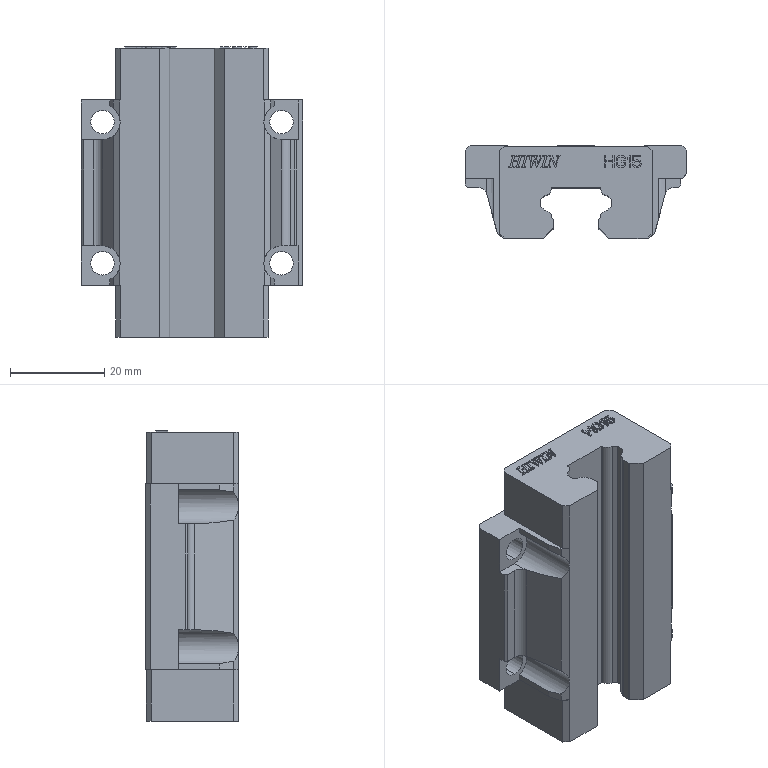Part | STEP file | 11-HGW1511 | 1 solid | 355 faces | box 47 x 19.7 x 61.7 mm | volume 35571 mm3 | plane 269 | spline 60 | cylinder 26 | commonest cylinder face diameters 0.8 x8 5 x8 3.24 x4 7.5 x4 4 x2